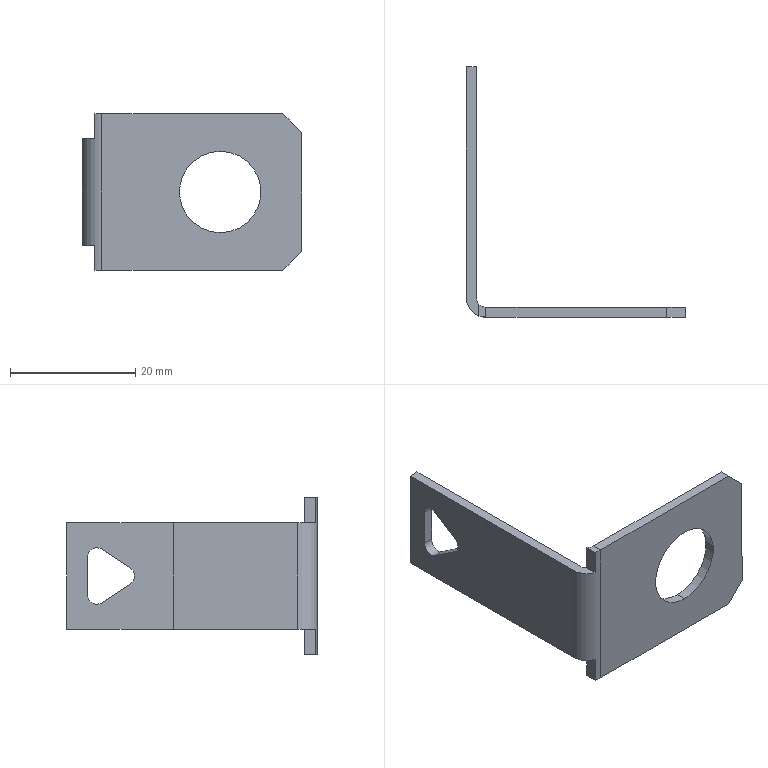Part | SolidWorks | features ICE 5, Chamfer 1, FlatPattern 1, SMBaseFlange 1, SheetMetal 1 | 1 solid | 31 faces | box 35 x 40 x 25 mm | volume 2088 mm3 | plane 23 | cylinder 8 | commonest cylinder face diameters 3 x5 13 x2 6.2 x1
STEP:
#1=CARTESIAN_POINT('',(22.,1.6,19.));
#2=VERTEX_POINT('',#1);
#3=CARTESIAN_POINT('',(22.,1.6,6.));
#4=VERTEX_POINT('',#3);
#5=CARTESIAN_POINT('',(22.,1.6,12.5));
#6=DIRECTION('',(0.,-1.,0.));
#7=DIRECTION('',(0.,0.,-1.));
#8=AXIS2_PLACEMENT_3D('',#5,#6,#7);
#9=CIRCLE('',#8,6.5);
#10=EDGE_CURVE('',#2,#4,#9,.T.);
#11=ORIENTED_EDGE('',*,*,#10,.F.);
#12=CARTESIAN_POINT('',(22.,0.,19.));
#13=VERTEX_POINT('',#12);
#14=CARTESIAN_POINT('',(22.,1.6,19.));
#15=DIRECTION('',(0.,-1.,0.));
#16=VECTOR('',#15,1000.);
#17=LINE('',#14,#16);
#18=EDGE_CURVE('',#2,#13,#17,.T.);
#19=ORIENTED_EDGE('',*,*,#18,.T.);
#20=CARTESIAN_POINT('',(22.,0.,6.));
#21=VERTEX_POINT('',#20);
#22=CARTESIAN_POINT('',(22.,0.,12.5));
#23=DIRECTION('',(0.,-1.,0.));
#24=DIRECTION('',(0.,0.,-1.));
#25=AXIS2_PLACEMENT_3D('',#22,#23,#24);
#26=CIRCLE('',#25,6.5);
#27=EDGE_CURVE('',#13,#21,#26,.T.);
#28=ORIENTED_EDGE('',*,*,#27,.T.);
#29=CARTESIAN_POINT('',(22.,1.6,6.));
#30=DIRECTION('',(0.,-1.,0.));
#31=VECTOR('',#30,1000.);
#32=LINE('',#29,#31);
#33=EDGE_CURVE('',#4,#21,#32,.T.);
#34=ORIENTED_EDGE('',*,*,#33,.F.);
#35=EDGE_LOOP('',(#11,#19,#28,#34));
#36=FACE_OUTER_BOUND('',#35,.T.);
#37=CARTESIAN_POINT('',(22.,1.6,12.5));
#38=DIRECTION('',(0.,-1.,0.));
#39=DIRECTION('',(0.,0.,-1.));
#40=AXIS2_PLACEMENT_3D('',#37,#38,#39);
#41=CYLINDRICAL_SURFACE('',#40,6.5);
#42=ADVANCED_FACE('',(#36),#41,.F.);
#43=CARTESIAN_POINT('',(1.59,29.204,12.5));
#44=VERTEX_POINT('',#43);
#45=CARTESIAN_POINT('',(1.59,29.872,13.748));
#46=VERTEX_POINT('',#45);
#47=CARTESIAN_POINT('',(1.59,30.704,12.5));
#48=DIRECTION('',(-1.,0.,0.));
#49=DIRECTION('',(0.,0.,-1.));
#50=AXIS2_PLACEMENT_3D('',#47,#48,#49);
#51=CIRCLE('',#50,1.5);
#52=EDGE_CURVE('',#44,#46,#51,.T.);
#53=ORIENTED_EDGE('',*,*,#52,.F.);
#54=CARTESIAN_POINT('',(0.01,29.204,12.5));
#55=VERTEX_POINT('',#54);
#56=CARTESIAN_POINT('',(1.6,29.204,12.5));
#57=DIRECTION('',(-1.,0.,0.));
#58=VECTOR('',#57,1000.);
#59=LINE('',#56,#58);
#60=EDGE_CURVE('',#44,#55,#59,.T.);
#61=ORIENTED_EDGE('',*,*,#60,.T.);
#62=CARTESIAN_POINT('',(0.01,29.872,13.748));
#63=VERTEX_POINT('',#62);
#64=CARTESIAN_POINT('',(0.01,30.704,12.5));
#65=DIRECTION('',(1.,0.,0.));
#66=DIRECTION('',(0.,0.,1.));
#67=AXIS2_PLACEMENT_3D('',#64,#65,#66);
#68=CIRCLE('',#67,1.5);
#69=EDGE_CURVE('',#63,#55,#68,.T.);
#70=ORIENTED_EDGE('',*,*,#69,.F.);
#71=CARTESIAN_POINT('',(1.6,29.872,13.748));
#72=DIRECTION('',(-1.,0.,0.));
#73=VECTOR('',#72,1000.);
#74=LINE('',#71,#73);
#75=EDGE_CURVE('',#46,#63,#74,.T.);
#76=ORIENTED_EDGE('',*,*,#75,.F.);
#77=EDGE_LOOP('',(#53,#61,#70,#76));
#78=FACE_OUTER_BOUND('',#77,.T.);
#79=CARTESIAN_POINT('',(1.6,30.704,12.5));
#80=DIRECTION('',(-1.,0.,0.));
#81=DIRECTION('',(0.,-1.,0.));
#82=AXIS2_PLACEMENT_3D('',#79,#80,#81);
#83=CYLINDRICAL_SURFACE('',#82,1.5);
#84=ADVANCED_FACE('',(#78),#83,.F.);
#85=CARTESIAN_POINT('',(1.59,40.,4.));
#86=VERTEX_POINT('',#85);
#87=CARTESIAN_POINT('',(0.01,40.,4.));
#88=VERTEX_POINT('',#87);
#89=CARTESIAN_POINT('',(2.,40.,4.));
#90=DIRECTION('',(-1.,0.,0.));
#91=VECTOR('',#90,1000.);
#92=LINE('',#89,#91);
#93=EDGE_CURVE('',#86,#88,#92,.T.);
#94=ORIENTED_EDGE('',*,*,#93,.T.);
#95=CARTESIAN_POINT('',(0.01,40.,21.));
#96=VERTEX_POINT('',#95);
#97=CARTESIAN_POINT('',(0.01,40.,4.));
#98=DIRECTION('',(0.,0.,-1.));
#99=VECTOR('',#98,1000.);
#100=LINE('',#97,#99);
#101=EDGE_CURVE('',#96,#88,#100,.T.);
#102=ORIENTED_EDGE('',*,*,#101,.F.);
#103=CARTESIAN_POINT('',(1.59,40.,21.));
#104=VERTEX_POINT('',#103);
#105=CARTESIAN_POINT('',(2.,40.,21.));
#106=DIRECTION('',(-1.,0.,0.));
#107=VECTOR('',#106,1000.);
#108=LINE('',#105,#107);
#109=EDGE_CURVE('',#104,#96,#108,.T.);
#110=ORIENTED_EDGE('',*,*,#109,.F.);
#111=CARTESIAN_POINT('',(1.59,40.,21.));
#112=DIRECTION('',(0.,0.,1.));
#113=VECTOR('',#112,1000.);
#114=LINE('',#111,#113);
#115=EDGE_CURVE('',#86,#104,#114,.T.);
#116=ORIENTED_EDGE('',*,*,#115,.F.);
#117=EDGE_LOOP('',(#94,#102,#110,#116));
#118=FACE_OUTER_BOUND('',#117,.T.);
#119=CARTESIAN_POINT('',(0.,40.,25.));
#120=DIRECTION('',(0.,1.,0.));
#121=DIRECTION('',(0.,0.,1.));
#122=AXIS2_PLACEMENT_3D('',#119,#120,#121);
#123=PLANE('',#122);
#124=ADVANCED_FACE('',(#118),#123,.T.);
#125=CARTESIAN_POINT('',(0.01,36.7,15.497));
#126=VERTEX_POINT('',#125);
#127=CARTESIAN_POINT('',(0.01,34.368,16.745));
#128=VERTEX_POINT('',#127);
#129=CARTESIAN_POINT('',(0.01,35.2,15.497));
#130=DIRECTION('',(1.,0.,0.));
#131=DIRECTION('',(0.,0.,1.));
#132=AXIS2_PLACEMENT_3D('',#129,#130,#131);
#133=CIRCLE('',#132,1.5);
#134=EDGE_CURVE('',#126,#128,#133,.T.);
#135=ORIENTED_EDGE('',*,*,#134,.F.);
#136=CARTESIAN_POINT('',(1.59,36.7,15.497));
#137=VERTEX_POINT('',#136);
#138=CARTESIAN_POINT('',(1.6,36.7,15.497));
#139=DIRECTION('',(-1.,0.,0.));
#140=VECTOR('',#139,1000.);
#141=LINE('',#138,#140);
#142=EDGE_CURVE('',#137,#126,#141,.T.);
#143=ORIENTED_EDGE('',*,*,#142,.F.);
#144=CARTESIAN_POINT('',(1.59,34.368,16.745));
#145=VERTEX_POINT('',#144);
#146=CARTESIAN_POINT('',(1.59,35.2,15.497));
#147=DIRECTION('',(-1.,0.,0.));
#148=DIRECTION('',(0.,0.,-1.));
#149=AXIS2_PLACEMENT_3D('',#146,#147,#148);
#150=CIRCLE('',#149,1.5);
#151=EDGE_CURVE('',#145,#137,#150,.T.);
#152=ORIENTED_EDGE('',*,*,#151,.F.);
#153=CARTESIAN_POINT('',(1.6,34.368,16.745));
#154=DIRECTION('',(-1.,0.,0.));
#155=VECTOR('',#154,1000.);
#156=LINE('',#153,#155);
#157=EDGE_CURVE('',#145,#128,#156,.T.);
#158=ORIENTED_EDGE('',*,*,#157,.T.);
#159=EDGE_LOOP('',(#135,#143,#152,#158));
#160=FACE_OUTER_BOUND('',#159,.T.);
#161=CARTESIAN_POINT('',(1.6,35.2,15.497));
#162=DIRECTION('',(-1.,0.,0.));
#163=DIRECTION('',(0.,-1.,0.));
#164=AXIS2_PLACEMENT_3D('',#161,#162,#163);
#165=CYLINDRICAL_SURFACE('',#164,1.5);
#166=ADVANCED_FACE('',(#160),#165,.F.);
#167=CARTESIAN_POINT('',(0.01,34.368,16.745));
#168=DIRECTION('',(0.,-0.8321,-0.5547));
#169=VECTOR('',#168,1000.);
#170=LINE('',#167,#169);
#171=EDGE_CURVE('',#128,#63,#170,.T.);
#172=ORIENTED_EDGE('',*,*,#171,.F.);
#173=ORIENTED_EDGE('',*,*,#157,.F.);
#174=CARTESIAN_POINT('',(1.59,34.368,16.745));
#175=DIRECTION('',(0.,0.8321,0.5547));
#176=VECTOR('',#175,1000.);
#177=LINE('',#174,#176);
#178=EDGE_CURVE('',#46,#145,#177,.T.);
#179=ORIENTED_EDGE('',*,*,#178,.F.);
#180=ORIENTED_EDGE('',*,*,#75,.T.);
#181=EDGE_LOOP('',(#172,#173,#179,#180));
#182=FACE_OUTER_BOUND('',#181,.T.);
#183=CARTESIAN_POINT('',(1.6,34.368,16.745));
#184=DIRECTION('',(0.,-0.5547,0.8321));
#185=DIRECTION('',(0.,-0.8321,-0.5547));
#186=AXIS2_PLACEMENT_3D('',#183,#184,#185);
#187=PLANE('',#186);
#188=ADVANCED_FACE('',(#182),#187,.F.);
#189=ORIENTED_EDGE('',*,*,#60,.F.);
#190=CARTESIAN_POINT('',(1.59,29.872,11.252));
#191=VERTEX_POINT('',#190);
#192=CARTESIAN_POINT('',(1.59,30.704,12.5));
#193=DIRECTION('',(-1.,0.,0.));
#194=DIRECTION('',(0.,0.,-1.));
#195=AXIS2_PLACEMENT_3D('',#192,#193,#194);
#196=CIRCLE('',#195,1.5);
#197=EDGE_CURVE('',#191,#44,#196,.T.);
#198=ORIENTED_EDGE('',*,*,#197,.F.);
#199=CARTESIAN_POINT('',(0.01,29.872,11.252));
#200=VERTEX_POINT('',#199);
#201=CARTESIAN_POINT('',(1.6,29.872,11.252));
#202=DIRECTION('',(-1.,0.,0.));
#203=VECTOR('',#202,1000.);
#204=LINE('',#201,#203);
#205=EDGE_CURVE('',#191,#200,#204,.T.);
#206=ORIENTED_EDGE('',*,*,#205,.T.);
#207=CARTESIAN_POINT('',(0.01,30.704,12.5));
#208=DIRECTION('',(1.,0.,0.));
#209=DIRECTION('',(0.,0.,1.));
#210=AXIS2_PLACEMENT_3D('',#207,#208,#209);
#211=CIRCLE('',#210,1.5);
#212=EDGE_CURVE('',#55,#200,#211,.T.);
#213=ORIENTED_EDGE('',*,*,#212,.F.);
#214=EDGE_LOOP('',(#189,#198,#206,#213));
#215=FACE_OUTER_BOUND('',#214,.T.);
#216=CARTESIAN_POINT('',(1.6,30.704,12.5));
#217=DIRECTION('',(-1.,0.,0.));
#218=DIRECTION('',(0.,-1.,0.));
#219=AXIS2_PLACEMENT_3D('',#216,#217,#218);
#220=CYLINDRICAL_SURFACE('',#219,1.5);
#221=ADVANCED_FACE('',(#215),#220,.F.);
#222=CARTESIAN_POINT('',(0.01,34.368,8.255));
#223=VERTEX_POINT('',#222);
#224=CARTESIAN_POINT('',(0.01,34.368,8.255));
#225=DIRECTION('',(0.,0.8321,-0.5547));
#226=VECTOR('',#225,1000.);
#227=LINE('',#224,#226);
#228=EDGE_CURVE('',#200,#223,#227,.T.);
#229=ORIENTED_EDGE('',*,*,#228,.F.);
#230=ORIENTED_EDGE('',*,*,#205,.F.);
#231=CARTESIAN_POINT('',(1.59,34.368,8.255));
#232=VERTEX_POINT('',#231);
#233=CARTESIAN_POINT('',(1.59,34.368,8.255));
#234=DIRECTION('',(0.,-0.8321,0.5547));
#235=VECTOR('',#234,1000.);
#236=LINE('',#233,#235);
#237=EDGE_CURVE('',#232,#191,#236,.T.);
#238=ORIENTED_EDGE('',*,*,#237,.F.);
#239=CARTESIAN_POINT('',(1.6,34.368,8.255));
#240=DIRECTION('',(-1.,0.,0.));
#241=VECTOR('',#240,1000.);
#242=LINE('',#239,#241);
#243=EDGE_CURVE('',#232,#223,#242,.T.);
#244=ORIENTED_EDGE('',*,*,#243,.T.);
#245=EDGE_LOOP('',(#229,#230,#238,#244));
#246=FACE_OUTER_BOUND('',#245,.T.);
#247=CARTESIAN_POINT('',(1.6,34.368,8.255));
#248=DIRECTION('',(0.,-0.5547,-0.8321));
#249=DIRECTION('',(0.,0.8321,-0.5547));
#250=AXIS2_PLACEMENT_3D('',#247,#248,#249);
#251=PLANE('',#250);
#252=ADVANCED_FACE('',(#246),#251,.F.);
#253=CARTESIAN_POINT('',(0.01,36.7,9.503));
#254=VERTEX_POINT('',#253);
#255=CARTESIAN_POINT('',(0.01,35.2,9.503));
#256=DIRECTION('',(1.,0.,0.));
#257=DIRECTION('',(0.,0.,1.));
#258=AXIS2_PLACEMENT_3D('',#255,#256,#257);
#259=CIRCLE('',#258,1.5);
#260=EDGE_CURVE('',#223,#254,#259,.T.);
#261=ORIENTED_EDGE('',*,*,#260,.F.);
#262=ORIENTED_EDGE('',*,*,#243,.F.);
#263=CARTESIAN_POINT('',(1.59,36.7,9.503));
#264=VERTEX_POINT('',#263);
#265=CARTESIAN_POINT('',(1.59,35.2,9.503));
#266=DIRECTION('',(-1.,0.,0.));
#267=DIRECTION('',(0.,0.,-1.));
#268=AXIS2_PLACEMENT_3D('',#265,#266,#267);
#269=CIRCLE('',#268,1.5);
#270=EDGE_CURVE('',#264,#232,#269,.T.);
#271=ORIENTED_EDGE('',*,*,#270,.F.);
#272=CARTESIAN_POINT('',(1.6,36.7,9.503));
#273=DIRECTION('',(-1.,0.,0.));
#274=VECTOR('',#273,1000.);
#275=LINE('',#272,#274);
#276=EDGE_CURVE('',#264,#254,#275,.T.);
#277=ORIENTED_EDGE('',*,*,#276,.T.);
#278=EDGE_LOOP('',(#261,#262,#271,#277));
#279=FACE_OUTER_BOUND('',#278,.T.);
#280=CARTESIAN_POINT('',(1.6,35.2,9.503));
#281=DIRECTION('',(-1.,0.,0.));
#282=DIRECTION('',(0.,-1.,0.));
#283=AXIS2_PLACEMENT_3D('',#280,#281,#282);
#284=CYLINDRICAL_SURFACE('',#283,1.5);
#285=ADVANCED_FACE('',(#279),#284,.F.);
#286=CARTESIAN_POINT('',(0.01,36.7,12.5));
#287=DIRECTION('',(0.,0.,1.));
#288=VECTOR('',#287,1000.);
#289=LINE('',#286,#288);
#290=EDGE_CURVE('',#254,#126,#289,.T.);
#291=ORIENTED_EDGE('',*,*,#290,.F.);
#292=ORIENTED_EDGE('',*,*,#276,.F.);
#293=CARTESIAN_POINT('',(1.59,36.7,12.5));
#294=DIRECTION('',(0.,0.,-1.));
#295=VECTOR('',#294,1000.);
#296=LINE('',#293,#295);
#297=EDGE_CURVE('',#137,#264,#296,.T.);
#298=ORIENTED_EDGE('',*,*,#297,.F.);
#299=ORIENTED_EDGE('',*,*,#142,.T.);
#300=EDGE_LOOP('',(#291,#292,#298,#299));
#301=FACE_OUTER_BOUND('',#300,.T.);
#302=CARTESIAN_POINT('',(1.6,36.7,12.5));
#303=DIRECTION('',(0.,1.,0.));
#304=DIRECTION('',(-1.,0.,0.));
#305=AXIS2_PLACEMENT_3D('',#302,#303,#304);
#306=PLANE('',#305);
#307=ADVANCED_FACE('',(#301),#306,.F.);
#308=CARTESIAN_POINT('',(2.,0.2017,0.));
#309=VERTEX_POINT('',#308);
#310=CARTESIAN_POINT('',(3.1,0.,0.));
#311=VERTEX_POINT('',#310);
#312=CARTESIAN_POINT('',(3.1,3.1,0.));
#313=DIRECTION('',(0.,0.,1.));
#314=DIRECTION('',(-1.,0.,0.));
#315=AXIS2_PLACEMENT_3D('',#312,#313,#314);
#316=CIRCLE('',#315,3.1);
#317=EDGE_CURVE('',#309,#311,#316,.T.);
#318=ORIENTED_EDGE('',*,*,#317,.F.);
#319=CARTESIAN_POINT('',(2.,2.08,0.));
#320=VERTEX_POINT('',#319);
#321=CARTESIAN_POINT('',(2.,0.,0.));
#322=DIRECTION('',(0.,1.,0.));
#323=VECTOR('',#322,1000.);
#324=LINE('',#321,#323);
#325=EDGE_CURVE('',#309,#320,#324,.T.);
#326=ORIENTED_EDGE('',*,*,#325,.T.);
#327=CARTESIAN_POINT('',(3.1,1.6,0.));
#328=VERTEX_POINT('',#327);
#329=CARTESIAN_POINT('',(3.1,3.1,0.));
#330=DIRECTION('',(0.,0.,1.));
#331=DIRECTION('',(1.,0.,0.));
#332=AXIS2_PLACEMENT_3D('',#329,#330,#331);
#333=CIRCLE('',#332,1.5);
#334=EDGE_CURVE('',#320,#328,#333,.T.);
#335=ORIENTED_EDGE('',*,*,#334,.T.);
#336=CARTESIAN_POINT('',(3.1,0.,0.));
#337=DIRECTION('',(0.,1.,0.));
#338=VECTOR('',#337,1000.);
#339=LINE('',#336,#338);
#340=EDGE_CURVE('',#311,#328,#339,.T.);
#341=ORIENTED_EDGE('',*,*,#340,.F.);
#342=EDGE_LOOP('',(#318,#326,#335,#341));
#343=FACE_OUTER_BOUND('',#342,.T.);
#344=CARTESIAN_POINT('',(3.1,0.,0.));
#345=DIRECTION('',(0.,0.,-1.));
#346=DIRECTION('',(-1.,0.,0.));
#347=AXIS2_PLACEMENT_3D('',#344,#345,#346);
#348=PLANE('',#347);
#349=ADVANCED_FACE('',(#343),#348,.T.);
#350=CARTESIAN_POINT('',(2.,0.2017,25.));
#351=VERTEX_POINT('',#350);
#352=CARTESIAN_POINT('',(2.,2.08,25.));
#353=VERTEX_POINT('',#352);
#354=CARTESIAN_POINT('',(2.,3.1,25.));
#355=DIRECTION('',(0.,1.,0.));
#356=VECTOR('',#355,1000.);
#357=LINE('',#354,#356);
#358=EDGE_CURVE('',#351,#353,#357,.T.);
#359=ORIENTED_EDGE('',*,*,#358,.F.);
#360=CARTESIAN_POINT('',(3.1,0.,25.));
#361=VERTEX_POINT('',#360);
#362=CARTESIAN_POINT('',(3.1,3.1,25.));
#363=DIRECTION('',(0.,0.,1.));
#364=DIRECTION('',(-1.,0.,0.));
#365=AXIS2_PLACEMENT_3D('',#362,#363,#364);
#366=CIRCLE('',#365,3.1);
#367=EDGE_CURVE('',#351,#361,#366,.T.);
#368=ORIENTED_EDGE('',*,*,#367,.T.);
#369=CARTESIAN_POINT('',(3.1,1.6,25.));
#370=VERTEX_POINT('',#369);
#371=CARTESIAN_POINT('',(3.1,1.6,25.));
#372=DIRECTION('',(0.,-1.,0.));
#373=VECTOR('',#372,1000.);
#374=LINE('',#371,#373);
#375=EDGE_CURVE('',#370,#361,#374,.T.);
#376=ORIENTED_EDGE('',*,*,#375,.F.);
#377=CARTESIAN_POINT('',(3.1,3.1,25.));
#378=DIRECTION('',(0.,0.,1.));
#379=DIRECTION('',(1.,0.,0.));
#380=AXIS2_PLACEMENT_3D('',#377,#378,#379);
#381=CIRCLE('',#380,1.5);
#382=EDGE_CURVE('',#353,#370,#381,.T.);
#383=ORIENTED_EDGE('',*,*,#382,.F.);
#384=EDGE_LOOP('',(#359,#368,#376,#383));
#385=FACE_OUTER_BOUND('',#384,.T.);
#386=CARTESIAN_POINT('',(0.,3.1,25.));
#387=DIRECTION('',(0.,0.,1.));
#388=DIRECTION('',(1.,0.,0.));
#389=AXIS2_PLACEMENT_3D('',#386,#387,#388);
#390=PLANE('',#389);
#391=ADVANCED_FACE('',(#385),#390,.T.);
#392=CARTESIAN_POINT('',(32.,1.6,0.));
#393=VERTEX_POINT('',#392);
#394=CARTESIAN_POINT('',(3.1,1.6,0.));
#395=DIRECTION('',(1.,0.,0.));
#396=VECTOR('',#395,1000.);
#397=LINE('',#394,#396);
#398=EDGE_CURVE('',#328,#393,#397,.T.);
#399=ORIENTED_EDGE('',*,*,#398,.T.);
#400=CARTESIAN_POINT('',(32.,0.,0.));
#401=VERTEX_POINT('',#400);
#402=CARTESIAN_POINT('',(32.,3.1,0.));
#403=DIRECTION('',(0.,-1.,0.));
#404=VECTOR('',#403,1000.);
#405=LINE('',#402,#404);
#406=EDGE_CURVE('',#393,#401,#405,.T.);
#407=ORIENTED_EDGE('',*,*,#406,.T.);
#408=CARTESIAN_POINT('',(3.1,0.,0.));
#409=DIRECTION('',(1.,0.,0.));
#410=VECTOR('',#409,1000.);
#411=LINE('',#408,#410);
#412=EDGE_CURVE('',#311,#401,#411,.T.);
#413=ORIENTED_EDGE('',*,*,#412,.F.);
#414=ORIENTED_EDGE('',*,*,#340,.T.);
#415=EDGE_LOOP('',(#399,#407,#413,#414));
#416=FACE_OUTER_BOUND('',#415,.T.);
#417=CARTESIAN_POINT('',(1.6,3.1,0.));
#418=DIRECTION('',(0.,0.,-1.));
#419=DIRECTION('',(-1.,0.,0.));
#420=AXIS2_PLACEMENT_3D('',#417,#418,#419);
#421=PLANE('',#420);
#422=ADVANCED_FACE('',(#416),#421,.T.);
#423=CARTESIAN_POINT('',(22.,0.,12.5));
#424=DIRECTION('',(0.,-1.,0.));
#425=DIRECTION('',(0.,0.,-1.));
#426=AXIS2_PLACEMENT_3D('',#423,#424,#425);
#427=CIRCLE('',#426,6.5);
#428=EDGE_CURVE('',#21,#13,#427,.T.);
#429=ORIENTED_EDGE('',*,*,#428,.F.);
#430=ORIENTED_EDGE('',*,*,#27,.F.);
#431=EDGE_LOOP('',(#429,#430));
#432=FACE_BOUND('',#431,.T.);
#433=ORIENTED_EDGE('',*,*,#412,.T.);
#434=CARTESIAN_POINT('',(35.,0.,3.));
#435=VERTEX_POINT('',#434);
#436=CARTESIAN_POINT('',(32.,0.,0.));
#437=DIRECTION('',(0.7071,0.,0.7071));
#438=VECTOR('',#437,1000.);
#439=LINE('',#436,#438);
#440=EDGE_CURVE('',#401,#435,#439,.T.);
#441=ORIENTED_EDGE('',*,*,#440,.T.);
#442=CARTESIAN_POINT('',(35.,0.,22.));
#443=VERTEX_POINT('',#442);
#444=CARTESIAN_POINT('',(35.,0.,25.));
#445=DIRECTION('',(0.,0.,-1.));
#446=VECTOR('',#445,1000.);
#447=LINE('',#444,#446);
#448=EDGE_CURVE('',#443,#435,#447,.T.);
#449=ORIENTED_EDGE('',*,*,#448,.F.);
#450=CARTESIAN_POINT('',(32.,0.,25.));
#451=VERTEX_POINT('',#450);
#452=CARTESIAN_POINT('',(35.,0.,22.));
#453=DIRECTION('',(-0.7071,0.,0.7071));
#454=VECTOR('',#453,1000.);
#455=LINE('',#452,#454);
#456=EDGE_CURVE('',#443,#451,#455,.T.);
#457=ORIENTED_EDGE('',*,*,#456,.T.);
#458=CARTESIAN_POINT('',(3.1,0.,25.));
#459=DIRECTION('',(1.,0.,0.));
#460=VECTOR('',#459,1000.);
#461=LINE('',#458,#460);
#462=EDGE_CURVE('',#361,#451,#461,.T.);
#463=ORIENTED_EDGE('',*,*,#462,.F.);
#464=CARTESIAN_POINT('',(3.1,0.,25.));
#465=DIRECTION('',(0.,0.,-1.));
#466=VECTOR('',#465,1000.);
#467=LINE('',#464,#466);
#468=EDGE_CURVE('',#361,#311,#467,.T.);
#469=ORIENTED_EDGE('',*,*,#468,.T.);
#470=EDGE_LOOP('',(#433,#441,#449,#457,#463,#469));
#471=FACE_OUTER_BOUND('',#470,.T.);
#472=CARTESIAN_POINT('',(3.1,0.,25.));
#473=DIRECTION('',(0.,1.,0.));
#474=DIRECTION('',(0.,0.,1.));
#475=AXIS2_PLACEMENT_3D('',#472,#473,#474);
#476=PLANE('',#475);
#477=ADVANCED_FACE('',(#432,#471),#476,.F.);
#478=ORIENTED_EDGE('',*,*,#448,.T.);
#479=CARTESIAN_POINT('',(35.,1.6,3.));
#480=VERTEX_POINT('',#479);
#481=CARTESIAN_POINT('',(35.,1.6,3.));
#482=DIRECTION('',(0.,1.,0.));
#483=VECTOR('',#482,1000.);
#484=LINE('',#481,#483);
#485=EDGE_CURVE('',#435,#480,#484,.T.);
#486=ORIENTED_EDGE('',*,*,#485,.T.);
#487=CARTESIAN_POINT('',(35.,1.6,22.));
#488=VERTEX_POINT('',#487);
#489=CARTESIAN_POINT('',(35.,1.6,25.));
#490=DIRECTION('',(0.,0.,-1.));
#491=VECTOR('',#490,1000.);
#492=LINE('',#489,#491);
#493=EDGE_CURVE('',#488,#480,#492,.T.);
#494=ORIENTED_EDGE('',*,*,#493,.F.);
#495=CARTESIAN_POINT('',(35.,1.6,22.));
#496=DIRECTION('',(0.,-1.,0.));
#497=VECTOR('',#496,1000.);
#498=LINE('',#495,#497);
#499=EDGE_CURVE('',#488,#443,#498,.T.);
#500=ORIENTED_EDGE('',*,*,#499,.T.);
#501=EDGE_LOOP('',(#478,#486,#494,#500));
#502=FACE_OUTER_BOUND('',#501,.T.);
#503=CARTESIAN_POINT('',(35.,1.6,25.));
#504=DIRECTION('',(1.,0.,0.));
#505=DIRECTION('',(0.,0.,-1.));
#506=AXIS2_PLACEMENT_3D('',#503,#504,#505);
#507=PLANE('',#506);
#508=ADVANCED_FACE('',(#502),#507,.T.);
#509=CARTESIAN_POINT('',(22.,1.6,12.5));
#510=DIRECTION('',(0.,-1.,0.));
#511=DIRECTION('',(0.,0.,-1.));
#512=AXIS2_PLACEMENT_3D('',#509,#510,#511);
#513=CIRCLE('',#512,6.5);
#514=EDGE_CURVE('',#4,#2,#513,.T.);
#515=ORIENTED_EDGE('',*,*,#514,.T.);
#516=ORIENTED_EDGE('',*,*,#10,.T.);
#517=EDGE_LOOP('',(#515,#516));
#518=FACE_BOUND('',#517,.T.);
#519=ORIENTED_EDGE('',*,*,#493,.T.);
#520=CARTESIAN_POINT('',(30.05,1.6,-1.95));
#521=DIRECTION('',(-0.7071,0.,-0.7071));
#522=VECTOR('',#521,1000.);
#523=LINE('',#520,#522);
#524=EDGE_CURVE('',#480,#393,#523,.T.);
#525=ORIENTED_EDGE('',*,*,#524,.T.);
#526=ORIENTED_EDGE('',*,*,#398,.F.);
#527=CARTESIAN_POINT('',(3.1,1.6,25.));
#528=DIRECTION('',(0.,0.,-1.));
#529=VECTOR('',#528,1000.);
#530=LINE('',#527,#529);
#531=EDGE_CURVE('',#370,#328,#530,.T.);
#532=ORIENTED_EDGE('',*,*,#531,.F.);
#533=CARTESIAN_POINT('',(32.,1.6,25.));
#534=VERTEX_POINT('',#533);
#535=CARTESIAN_POINT('',(3.1,1.6,25.));
#536=DIRECTION('',(1.,0.,0.));
#537=VECTOR('',#536,1000.);
#538=LINE('',#535,#537);
#539=EDGE_CURVE('',#370,#534,#538,.T.);
#540=ORIENTED_EDGE('',*,*,#539,.T.);
#541=CARTESIAN_POINT('',(17.55,1.6,39.45));
#542=DIRECTION('',(0.7071,0.,-0.7071));
#543=VECTOR('',#542,1000.);
#544=LINE('',#541,#543);
#545=EDGE_CURVE('',#534,#488,#544,.T.);
#546=ORIENTED_EDGE('',*,*,#545,.T.);
#547=EDGE_LOOP('',(#519,#525,#526,#532,#540,#546));
#548=FACE_OUTER_BOUND('',#547,.T.);
#549=CARTESIAN_POINT('',(3.1,1.6,25.));
#550=DIRECTION('',(0.,1.,0.));
#551=DIRECTION('',(0.,0.,1.));
#552=AXIS2_PLACEMENT_3D('',#549,#550,#551);
#553=PLANE('',#552);
#554=ADVANCED_FACE('',(#518,#548),#553,.T.);
#555=CARTESIAN_POINT('',(1.6,3.1,4.));
#556=VERTEX_POINT('',#555);
#557=CARTESIAN_POINT('',(2.,2.08,4.));
#558=VERTEX_POINT('',#557);
#559=CARTESIAN_POINT('',(3.1,3.1,4.));
#560=DIRECTION('',(0.,0.,1.));
#561=DIRECTION('',(1.,0.,0.));
#562=AXIS2_PLACEMENT_3D('',#559,#560,#561);
#563=CIRCLE('',#562,1.5);
#564=EDGE_CURVE('',#556,#558,#563,.T.);
#565=ORIENTED_EDGE('',*,*,#564,.F.);
#566=CARTESIAN_POINT('',(1.6,3.1,21.));
#567=VERTEX_POINT('',#566);
#568=CARTESIAN_POINT('',(1.6,3.1,25.));
#569=DIRECTION('',(0.,0.,-1.));
#570=VECTOR('',#569,1000.);
#571=LINE('',#568,#570);
#572=EDGE_CURVE('',#567,#556,#571,.T.);
#573=ORIENTED_EDGE('',*,*,#572,.F.);
#574=CARTESIAN_POINT('',(2.,2.08,21.));
#575=VERTEX_POINT('',#574);
#576=CARTESIAN_POINT('',(3.1,3.1,21.));
#577=DIRECTION('',(0.,0.,-1.));
#578=DIRECTION('',(-1.,0.,0.));
#579=AXIS2_PLACEMENT_3D('',#576,#577,#578);
#580=CIRCLE('',#579,1.5);
#581=EDGE_CURVE('',#575,#567,#580,.T.);
#582=ORIENTED_EDGE('',*,*,#581,.F.);
#583=CARTESIAN_POINT('',(2.,2.08,25.));
#584=DIRECTION('',(0.,0.,-1.));
#585=VECTOR('',#584,1000.);
#586=LINE('',#583,#585);
#587=EDGE_CURVE('',#353,#575,#586,.T.);
#588=ORIENTED_EDGE('',*,*,#587,.F.);
#589=ORIENTED_EDGE('',*,*,#382,.T.);
#590=ORIENTED_EDGE('',*,*,#531,.T.);
#591=ORIENTED_EDGE('',*,*,#334,.F.);
#592=CARTESIAN_POINT('',(2.,2.08,25.));
#593=DIRECTION('',(0.,0.,1.));
#594=VECTOR('',#593,1000.);
#595=LINE('',#592,#594);
#596=EDGE_CURVE('',#320,#558,#595,.T.);
#597=ORIENTED_EDGE('',*,*,#596,.T.);
#598=EDGE_LOOP('',(#565,#573,#582,#588,#589,#590,#591,#597));
#599=FACE_OUTER_BOUND('',#598,.T.);
#600=CARTESIAN_POINT('',(3.1,3.1,25.));
#601=DIRECTION('',(0.,0.,-1.));
#602=DIRECTION('',(-1.,0.,0.));
#603=AXIS2_PLACEMENT_3D('',#600,#601,#602);
#604=CYLINDRICAL_SURFACE('',#603,1.5);
#605=ADVANCED_FACE('',(#599),#604,.F.);
#606=CARTESIAN_POINT('',(1.6,23.,21.));
#607=VERTEX_POINT('',#606);
#608=CARTESIAN_POINT('',(1.6,23.,4.));
#609=VERTEX_POINT('',#608);
#610=CARTESIAN_POINT('',(1.6,23.,21.));
#611=DIRECTION('',(0.,0.,-1.));
#612=VECTOR('',#611,1000.);
#613=LINE('',#610,#612);
#614=EDGE_CURVE('',#607,#609,#613,.T.);
#615=ORIENTED_EDGE('',*,*,#614,.F.);
#616=CARTESIAN_POINT('',(1.6,40.,21.));
#617=DIRECTION('',(0.,1.,0.));
#618=VECTOR('',#617,1000.);
#619=LINE('',#616,#618);
#620=EDGE_CURVE('',#567,#607,#619,.T.);
#621=ORIENTED_EDGE('',*,*,#620,.F.);
#622=ORIENTED_EDGE('',*,*,#572,.T.);
#623=CARTESIAN_POINT('',(1.6,40.,4.));
#624=DIRECTION('',(0.,-1.,0.));
#625=VECTOR('',#624,1000.);
#626=LINE('',#623,#625);
#627=EDGE_CURVE('',#609,#556,#626,.T.);
#628=ORIENTED_EDGE('',*,*,#627,.F.);
#629=EDGE_LOOP('',(#615,#621,#622,#628));
#630=FACE_OUTER_BOUND('',#629,.T.);
#631=CARTESIAN_POINT('',(1.6,40.,25.));
#632=DIRECTION('',(1.,0.,0.));
#633=DIRECTION('',(0.,1.,0.));
#634=AXIS2_PLACEMENT_3D('',#631,#632,#633);
#635=PLANE('',#634);
#636=ADVANCED_FACE('',(#630),#635,.T.);
#637=CARTESIAN_POINT('',(0.,23.,21.));
#638=VERTEX_POINT('',#637);
#639=CARTESIAN_POINT('',(0.,3.1,21.));
#640=VERTEX_POINT('',#639);
#641=CARTESIAN_POINT('',(0.,-7.015,21.));
#642=DIRECTION('',(0.,-1.,0.));
#643=VECTOR('',#642,1000.);
#644=LINE('',#641,#643);
#645=EDGE_CURVE('',#638,#640,#644,.T.);
#646=ORIENTED_EDGE('',*,*,#645,.F.);
#647=CARTESIAN_POINT('',(0.,23.,4.));
#648=VERTEX_POINT('',#647);
#649=CARTESIAN_POINT('',(0.,23.,4.));
#650=DIRECTION('',(0.,0.,1.));
#651=VECTOR('',#650,1000.);
#652=LINE('',#649,#651);
#653=EDGE_CURVE('',#648,#638,#652,.T.);
#654=ORIENTED_EDGE('',*,*,#653,.F.);
#655=CARTESIAN_POINT('',(0.,3.1,4.));
#656=VERTEX_POINT('',#655);
#657=CARTESIAN_POINT('',(0.,40.,4.));
#658=DIRECTION('',(0.,1.,0.));
#659=VECTOR('',#658,1000.);
#660=LINE('',#657,#659);
#661=EDGE_CURVE('',#656,#648,#660,.T.);
#662=ORIENTED_EDGE('',*,*,#661,.F.);
#663=CARTESIAN_POINT('',(0.,3.1,25.));
#664=DIRECTION('',(0.,0.,-1.));
#665=VECTOR('',#664,1000.);
#666=LINE('',#663,#665);
#667=EDGE_CURVE('',#640,#656,#666,.T.);
#668=ORIENTED_EDGE('',*,*,#667,.F.);
#669=EDGE_LOOP('',(#646,#654,#662,#668));
#670=FACE_OUTER_BOUND('',#669,.T.);
#671=CARTESIAN_POINT('',(0.,40.,25.));
#672=DIRECTION('',(1.,0.,0.));
#673=DIRECTION('',(0.,1.,0.));
#674=AXIS2_PLACEMENT_3D('',#671,#672,#673);
#675=PLANE('',#674);
#676=ADVANCED_FACE('',(#670),#675,.F.);
#677=ORIENTED_EDGE('',*,*,#667,.T.);
#678=CARTESIAN_POINT('',(2.,0.2017,4.));
#679=VERTEX_POINT('',#678);
#680=CARTESIAN_POINT('',(3.1,3.1,4.));
#681=DIRECTION('',(0.,0.,1.));
#682=DIRECTION('',(1.,0.,0.));
#683=AXIS2_PLACEMENT_3D('',#680,#681,#682);
#684=CIRCLE('',#683,3.1);
#685=EDGE_CURVE('',#656,#679,#684,.T.);
#686=ORIENTED_EDGE('',*,*,#685,.T.);
#687=CARTESIAN_POINT('',(2.,0.2017,25.));
#688=DIRECTION('',(0.,0.,1.));
#689=VECTOR('',#688,1000.);
#690=LINE('',#687,#689);
#691=EDGE_CURVE('',#309,#679,#690,.T.);
#692=ORIENTED_EDGE('',*,*,#691,.F.);
#693=ORIENTED_EDGE('',*,*,#317,.T.);
#694=ORIENTED_EDGE('',*,*,#468,.F.);
#695=ORIENTED_EDGE('',*,*,#367,.F.);
#696=CARTESIAN_POINT('',(2.,0.2017,21.));
#697=VERTEX_POINT('',#696);
#698=CARTESIAN_POINT('',(2.,0.2017,25.));
#699=DIRECTION('',(0.,0.,-1.));
#700=VECTOR('',#699,1000.);
#701=LINE('',#698,#700);
#702=EDGE_CURVE('',#351,#697,#701,.T.);
#703=ORIENTED_EDGE('',*,*,#702,.T.);
#704=CARTESIAN_POINT('',(3.1,3.1,21.));
#705=DIRECTION('',(0.,0.,-1.));
#706=DIRECTION('',(-1.,0.,0.));
#707=AXIS2_PLACEMENT_3D('',#704,#705,#706);
#708=CIRCLE('',#707,3.1);
#709=EDGE_CURVE('',#697,#640,#708,.T.);
#710=ORIENTED_EDGE('',*,*,#709,.T.);
#711=EDGE_LOOP('',(#677,#686,#692,#693,#694,#695,#703,#710));
#712=FACE_OUTER_BOUND('',#711,.T.);
#713=CARTESIAN_POINT('',(3.1,3.1,25.));
#714=DIRECTION('',(0.,0.,-1.));
#715=DIRECTION('',(-1.,0.,0.));
#716=AXIS2_PLACEMENT_3D('',#713,#714,#715);
#717=CYLINDRICAL_SURFACE('',#716,3.1);
#718=ADVANCED_FACE('',(#712),#717,.T.);
#719=ORIENTED_EDGE('',*,*,#462,.T.);
#720=CARTESIAN_POINT('',(32.,3.1,25.));
#721=DIRECTION('',(0.,1.,0.));
#722=VECTOR('',#721,1000.);
#723=LINE('',#720,#722);
#724=EDGE_CURVE('',#451,#534,#723,.T.);
#725=ORIENTED_EDGE('',*,*,#724,.T.);
#726=ORIENTED_EDGE('',*,*,#539,.F.);
#727=ORIENTED_EDGE('',*,*,#375,.T.);
#728=EDGE_LOOP('',(#719,#725,#726,#727));
#729=FACE_OUTER_BOUND('',#728,.T.);
#730=CARTESIAN_POINT('',(3.1,3.1,25.));
#731=DIRECTION('',(0.,0.,1.));
#732=DIRECTION('',(1.,0.,0.));
#733=AXIS2_PLACEMENT_3D('',#730,#731,#732);
#734=PLANE('',#733);
#735=ADVANCED_FACE('',(#729),#734,.T.);
#736=CARTESIAN_POINT('',(0.01,23.,21.));
#737=VERTEX_POINT('',#736);
#738=CARTESIAN_POINT('',(0.01,40.,21.));
#739=DIRECTION('',(0.,1.,0.));
#740=VECTOR('',#739,1000.);
#741=LINE('',#738,#740);
#742=EDGE_CURVE('',#737,#96,#741,.T.);
#743=ORIENTED_EDGE('',*,*,#742,.F.);
#744=CARTESIAN_POINT('',(0.01,23.,21.));
#745=DIRECTION('',(-1.,0.,0.));
#746=VECTOR('',#745,1000.);
#747=LINE('',#744,#746);
#748=EDGE_CURVE('',#737,#638,#747,.T.);
#749=ORIENTED_EDGE('',*,*,#748,.T.);
#750=ORIENTED_EDGE('',*,*,#645,.T.);
#751=ORIENTED_EDGE('',*,*,#709,.F.);
#752=CARTESIAN_POINT('',(2.,40.,21.));
#753=DIRECTION('',(0.,-1.,0.));
#754=VECTOR('',#753,1000.);
#755=LINE('',#752,#754);
#756=EDGE_CURVE('',#575,#697,#755,.T.);
#757=ORIENTED_EDGE('',*,*,#756,.F.);
#758=ORIENTED_EDGE('',*,*,#581,.T.);
#759=ORIENTED_EDGE('',*,*,#620,.T.);
#760=CARTESIAN_POINT('',(1.59,23.,21.));
#761=VERTEX_POINT('',#760);
#762=CARTESIAN_POINT('',(1.59,23.,21.));
#763=DIRECTION('',(1.,0.,0.));
#764=VECTOR('',#763,1000.);
#765=LINE('',#762,#764);
#766=EDGE_CURVE('',#761,#607,#765,.T.);
#767=ORIENTED_EDGE('',*,*,#766,.F.);
#768=CARTESIAN_POINT('',(1.59,40.,21.));
#769=DIRECTION('',(0.,-1.,0.));
#770=VECTOR('',#769,1000.);
#771=LINE('',#768,#770);
#772=EDGE_CURVE('',#104,#761,#771,.T.);
#773=ORIENTED_EDGE('',*,*,#772,.F.);
#774=ORIENTED_EDGE('',*,*,#109,.T.);
#775=EDGE_LOOP('',(#743,#749,#750,#751,#757,#758,#759,#767,#773,#774));
#776=FACE_OUTER_BOUND('',#775,.T.);
#777=CARTESIAN_POINT('',(2.,-7.015,21.));
#778=DIRECTION('',(0.,0.,-1.));
#779=DIRECTION('',(-1.,0.,0.));
#780=AXIS2_PLACEMENT_3D('',#777,#778,#779);
#781=PLANE('',#780);
#782=ADVANCED_FACE('',(#776),#781,.F.);
#783=ORIENTED_EDGE('',*,*,#587,.T.);
#784=ORIENTED_EDGE('',*,*,#756,.T.);
#785=ORIENTED_EDGE('',*,*,#702,.F.);
#786=ORIENTED_EDGE('',*,*,#358,.T.);
#787=EDGE_LOOP('',(#783,#784,#785,#786));
#788=FACE_OUTER_BOUND('',#787,.T.);
#789=CARTESIAN_POINT('',(2.,0.,0.));
#790=DIRECTION('',(1.,0.,0.));
#791=DIRECTION('',(0.,1.,0.));
#792=AXIS2_PLACEMENT_3D('',#789,#790,#791);
#793=PLANE('',#792);
#794=ADVANCED_FACE('',(#788),#793,.F.);
#795=ORIENTED_EDGE('',*,*,#661,.T.);
#796=CARTESIAN_POINT('',(0.01,23.,4.));
#797=VERTEX_POINT('',#796);
#798=CARTESIAN_POINT('',(0.01,23.,4.));
#799=DIRECTION('',(-1.,0.,0.));
#800=VECTOR('',#799,1000.);
#801=LINE('',#798,#800);
#802=EDGE_CURVE('',#797,#648,#801,.T.);
#803=ORIENTED_EDGE('',*,*,#802,.F.);
#804=CARTESIAN_POINT('',(0.01,40.,4.));
#805=DIRECTION('',(0.,-1.,0.));
#806=VECTOR('',#805,1000.);
#807=LINE('',#804,#806);
#808=EDGE_CURVE('',#88,#797,#807,.T.);
#809=ORIENTED_EDGE('',*,*,#808,.F.);
#810=ORIENTED_EDGE('',*,*,#93,.F.);
#811=CARTESIAN_POINT('',(1.59,23.,4.));
#812=VERTEX_POINT('',#811);
#813=CARTESIAN_POINT('',(1.59,40.,4.));
#814=DIRECTION('',(0.,1.,0.));
#815=VECTOR('',#814,1000.);
#816=LINE('',#813,#815);
#817=EDGE_CURVE('',#812,#86,#816,.T.);
#818=ORIENTED_EDGE('',*,*,#817,.F.);
#819=CARTESIAN_POINT('',(1.59,23.,4.));
#820=DIRECTION('',(1.,0.,0.));
#821=VECTOR('',#820,1000.);
#822=LINE('',#819,#821);
#823=EDGE_CURVE('',#812,#609,#822,.T.);
#824=ORIENTED_EDGE('',*,*,#823,.T.);
#825=ORIENTED_EDGE('',*,*,#627,.T.);
#826=ORIENTED_EDGE('',*,*,#564,.T.);
#827=CARTESIAN_POINT('',(2.,-5.077,4.));
#828=DIRECTION('',(0.,1.,0.));
#829=VECTOR('',#828,1000.);
#830=LINE('',#827,#829);
#831=EDGE_CURVE('',#679,#558,#830,.T.);
#832=ORIENTED_EDGE('',*,*,#831,.F.);
#833=ORIENTED_EDGE('',*,*,#685,.F.);
#834=EDGE_LOOP('',(#795,#803,#809,#810,#818,#824,#825,#826,#832,#833));
#835=FACE_OUTER_BOUND('',#834,.T.);
#836=CARTESIAN_POINT('',(2.,40.,4.));
#837=DIRECTION('',(0.,0.,1.));
#838=DIRECTION('',(1.,0.,0.));
#839=AXIS2_PLACEMENT_3D('',#836,#837,#838);
#840=PLANE('',#839);
#841=ADVANCED_FACE('',(#835),#840,.F.);
#842=ORIENTED_EDGE('',*,*,#325,.F.);
#843=ORIENTED_EDGE('',*,*,#691,.T.);
#844=ORIENTED_EDGE('',*,*,#831,.T.);
#845=ORIENTED_EDGE('',*,*,#596,.F.);
#846=EDGE_LOOP('',(#842,#843,#844,#845));
#847=FACE_OUTER_BOUND('',#846,.T.);
#848=CARTESIAN_POINT('',(2.,0.,0.));
#849=DIRECTION('',(-1.,0.,0.));
#850=DIRECTION('',(0.,-1.,0.));
#851=AXIS2_PLACEMENT_3D('',#848,#849,#850);
#852=PLANE('',#851);
#853=ADVANCED_FACE('',(#847),#852,.T.);
#854=ORIENTED_EDGE('',*,*,#18,.F.);
#855=ORIENTED_EDGE('',*,*,#514,.F.);
#856=ORIENTED_EDGE('',*,*,#33,.T.);
#857=ORIENTED_EDGE('',*,*,#428,.T.);
#858=EDGE_LOOP('',(#854,#855,#856,#857));
#859=FACE_OUTER_BOUND('',#858,.T.);
#860=CARTESIAN_POINT('',(22.,1.6,12.5));
#861=DIRECTION('',(0.,-1.,0.));
#862=DIRECTION('',(0.,0.,-1.));
#863=AXIS2_PLACEMENT_3D('',#860,#861,#862);
#864=CYLINDRICAL_SURFACE('',#863,6.5);
#865=ADVANCED_FACE('',(#859),#864,.F.);
#866=ORIENTED_EDGE('',*,*,#524,.F.);
#867=ORIENTED_EDGE('',*,*,#485,.F.);
#868=ORIENTED_EDGE('',*,*,#440,.F.);
#869=ORIENTED_EDGE('',*,*,#406,.F.);
#870=EDGE_LOOP('',(#866,#867,#868,#869));
#871=FACE_OUTER_BOUND('',#870,.T.);
#872=CARTESIAN_POINT('',(32.,3.1,0.));
#873=DIRECTION('',(-0.7071,0.,0.7071));
#874=DIRECTION('',(0.,-1.,0.));
#875=AXIS2_PLACEMENT_3D('',#872,#873,#874);
#876=PLANE('',#875);
#877=ADVANCED_FACE('',(#871),#876,.F.);
#878=ORIENTED_EDGE('',*,*,#545,.F.);
#879=ORIENTED_EDGE('',*,*,#724,.F.);
#880=ORIENTED_EDGE('',*,*,#456,.F.);
#881=ORIENTED_EDGE('',*,*,#499,.F.);
#882=EDGE_LOOP('',(#878,#879,#880,#881));
#883=FACE_OUTER_BOUND('',#882,.T.);
#884=CARTESIAN_POINT('',(35.,1.6,22.));
#885=DIRECTION('',(-0.7071,0.,-0.7071));
#886=DIRECTION('',(0.,-1.,0.));
#887=AXIS2_PLACEMENT_3D('',#884,#885,#886);
#888=PLANE('',#887);
#889=ADVANCED_FACE('',(#883),#888,.F.);
#890=ORIENTED_EDGE('',*,*,#772,.T.);
#891=CARTESIAN_POINT('',(1.59,23.,21.));
#892=DIRECTION('',(0.,0.,-1.));
#893=VECTOR('',#892,1000.);
#894=LINE('',#891,#893);
#895=EDGE_CURVE('',#761,#812,#894,.T.);
#896=ORIENTED_EDGE('',*,*,#895,.T.);
#897=ORIENTED_EDGE('',*,*,#817,.T.);
#898=ORIENTED_EDGE('',*,*,#115,.T.);
#899=EDGE_LOOP('',(#890,#896,#897,#898));
#900=FACE_OUTER_BOUND('',#899,.T.);
#901=ORIENTED_EDGE('',*,*,#151,.T.);
#902=ORIENTED_EDGE('',*,*,#297,.T.);
#903=ORIENTED_EDGE('',*,*,#270,.T.);
#904=ORIENTED_EDGE('',*,*,#237,.T.);
#905=ORIENTED_EDGE('',*,*,#197,.T.);
#906=ORIENTED_EDGE('',*,*,#52,.T.);
#907=ORIENTED_EDGE('',*,*,#178,.T.);
#908=EDGE_LOOP('',(#901,#902,#903,#904,#905,#906,#907));
#909=FACE_BOUND('',#908,.T.);
#910=CARTESIAN_POINT('',(1.59,0.,0.));
#911=DIRECTION('',(1.,0.,0.));
#912=DIRECTION('',(0.,0.,-1.));
#913=AXIS2_PLACEMENT_3D('',#910,#911,#912);
#914=PLANE('',#913);
#915=ADVANCED_FACE('',(#900,#909),#914,.T.);
#916=ORIENTED_EDGE('',*,*,#614,.T.);
#917=ORIENTED_EDGE('',*,*,#823,.F.);
#918=ORIENTED_EDGE('',*,*,#895,.F.);
#919=ORIENTED_EDGE('',*,*,#766,.T.);
#920=EDGE_LOOP('',(#916,#917,#918,#919));
#921=FACE_OUTER_BOUND('',#920,.T.);
#922=CARTESIAN_POINT('',(1.59,23.,21.));
#923=DIRECTION('',(0.,-1.,0.));
#924=DIRECTION('',(1.,0.,0.));
#925=AXIS2_PLACEMENT_3D('',#922,#923,#924);
#926=PLANE('',#925);
#927=ADVANCED_FACE('',(#921),#926,.F.);
#928=ORIENTED_EDGE('',*,*,#808,.T.);
#929=CARTESIAN_POINT('',(0.01,23.,4.));
#930=DIRECTION('',(0.,0.,1.));
#931=VECTOR('',#930,1000.);
#932=LINE('',#929,#931);
#933=EDGE_CURVE('',#797,#737,#932,.T.);
#934=ORIENTED_EDGE('',*,*,#933,.T.);
#935=ORIENTED_EDGE('',*,*,#742,.T.);
#936=ORIENTED_EDGE('',*,*,#101,.T.);
#937=EDGE_LOOP('',(#928,#934,#935,#936));
#938=FACE_OUTER_BOUND('',#937,.T.);
#939=ORIENTED_EDGE('',*,*,#134,.T.);
#940=ORIENTED_EDGE('',*,*,#171,.T.);
#941=ORIENTED_EDGE('',*,*,#69,.T.);
#942=ORIENTED_EDGE('',*,*,#212,.T.);
#943=ORIENTED_EDGE('',*,*,#228,.T.);
#944=ORIENTED_EDGE('',*,*,#260,.T.);
#945=ORIENTED_EDGE('',*,*,#290,.T.);
#946=EDGE_LOOP('',(#939,#940,#941,#942,#943,#944,#945));
#947=FACE_BOUND('',#946,.T.);
#948=CARTESIAN_POINT('',(0.01,0.,0.));
#949=DIRECTION('',(-1.,0.,0.));
#950=DIRECTION('',(0.,0.,1.));
#951=AXIS2_PLACEMENT_3D('',#948,#949,#950);
#952=PLANE('',#951);
#953=ADVANCED_FACE('',(#938,#947),#952,.T.);
#954=ORIENTED_EDGE('',*,*,#653,.T.);
#955=ORIENTED_EDGE('',*,*,#748,.F.);
#956=ORIENTED_EDGE('',*,*,#933,.F.);
#957=ORIENTED_EDGE('',*,*,#802,.T.);
#958=EDGE_LOOP('',(#954,#955,#956,#957));
#959=FACE_OUTER_BOUND('',#958,.T.);
#960=CARTESIAN_POINT('',(0.01,23.,4.));
#961=DIRECTION('',(0.,-1.,0.));
#962=DIRECTION('',(1.,0.,0.));
#963=AXIS2_PLACEMENT_3D('',#960,#961,#962);
#964=PLANE('',#963);
#965=ADVANCED_FACE('',(#959),#964,.F.);
#966=CLOSED_SHELL('',(#42,#84,#124,#166,#188,#221,#252,#285,#307,#349,#391,#422,#477,#508,#554,#605,#636,#676,#718,#735,#782,#794,#841,#853,#865,#877,#889,#915,#927,#953,#965));
#967=MANIFOLD_SOLID_BREP('',#966);
#968=CARTESIAN_POINT('',(0.,0.,0.));
#969=DIRECTION('',(0.,0.,1.));
#970=DIRECTION('',(1.,0.,0.));
#971=AXIS2_PLACEMENT_3D('',#968,#969,#970);
#972=(LENGTH_UNIT()NAMED_UNIT(*)SI_UNIT(.MILLI.,.METRE.));
#973=UNCERTAINTY_MEASURE_WITH_UNIT(LENGTH_MEASURE(0.00001),#972,'','');
#974=(NAMED_UNIT(*)PLANE_ANGLE_UNIT()SI_UNIT($,.RADIAN.));
#975=(NAMED_UNIT(*)SI_UNIT($,.STERADIAN.)SOLID_ANGLE_UNIT());
#976=(GEOMETRIC_REPRESENTATION_CONTEXT(3)GLOBAL_UNCERTAINTY_ASSIGNED_CONTEXT((#973))GLOBAL_UNIT_ASSIGNED_CONTEXT((#972,#974,#975))REPRESENTATION_CONTEXT('',''));
#977=ADVANCED_BREP_SHAPE_REPRESENTATION('',(#967,#971),#976);